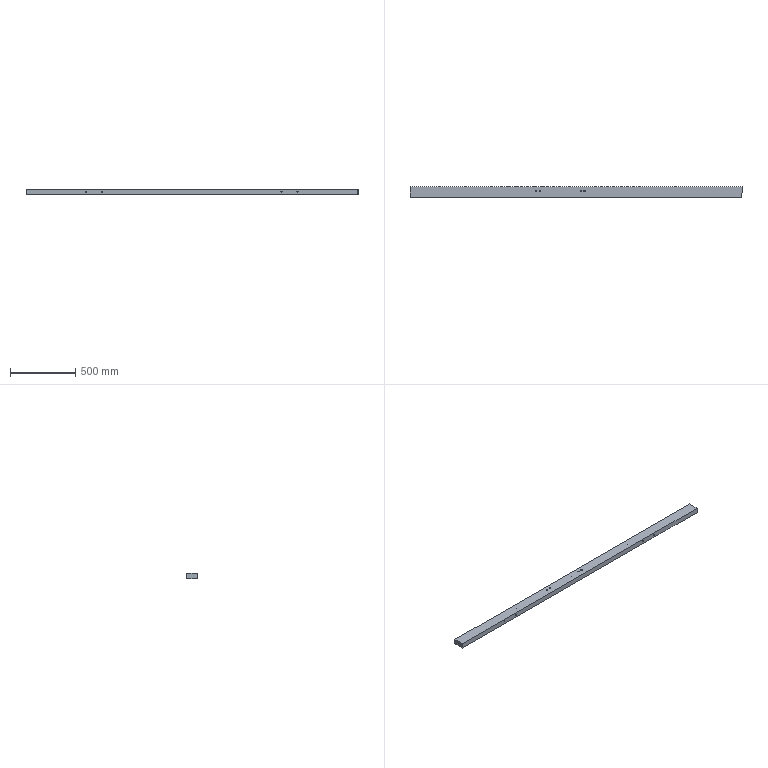Part | SolidWorks | features Cut 4, Extrusion 1, LPattern 1 | 1 solid | 96 faces | box 2544 x 80 x 40 mm | volume 8091371 mm3 | cylinder 60 | plane 36 | commonest cylinder face diameters 6.6 x20 6.671 x20 9 x8 10 x8 15 x4